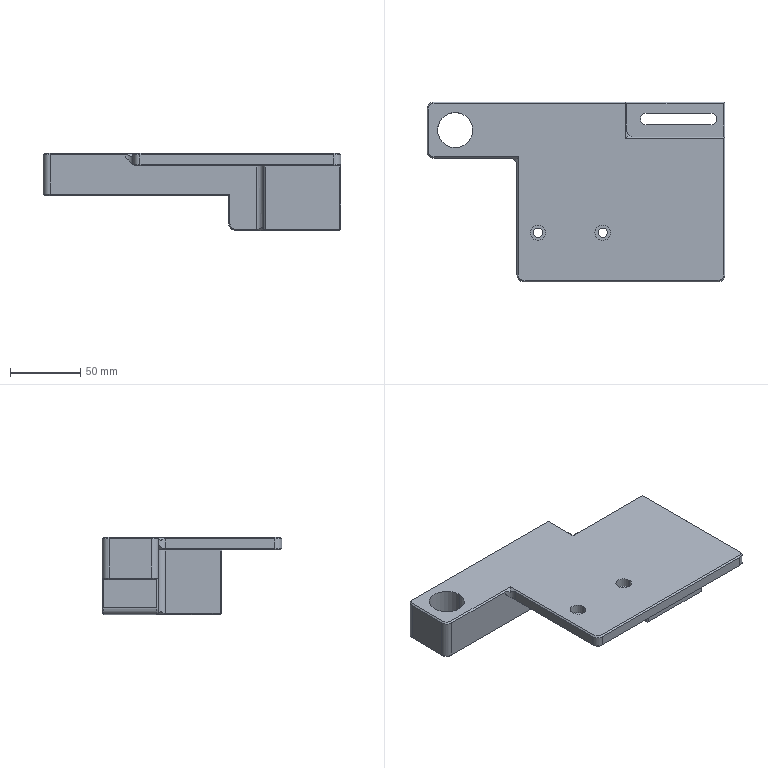NC program | NX | posted with a generic post | part box 212 x 128 x 55 mm
Lines 5359 to 7213 of 7327, first 1601 of 1847 lines:
(ZLEVEL_PROFILE_COPY_COPY_COPY , TOOL : D10)
N10674 T09 M6
N10676 G54
N10678 G17 G0 G90 X-48.2 Y14.719 S2000 M3
N10680 G43 Z30. H9
N10682 Z-0.2
N10684 G94 G1 X-46.7 Y15.585 F1000.
N10686 G3 X-46.2 Y16.451 R1.
N10688 G1 Y19.8 F2000.
N10690 X-49.549
N10692 G3 X-50.415 Y19.3 R1.
N10694 G1 X-51.281 Y17.8
N10696 G0 X-48.4 Y14.519 Z-0.4
N10698 G1 X-46.9 Y15.385 F1000.
N10700 G3 X-46.4 Y16.251 R1.
N10702 G1 Y19.6 F2000.
N10704 X-49.749
N10706 G3 X-50.615 Y19.1 R1.
N10708 G1 X-51.481 Y17.6
N10710 G0 X-48.6 Y14.319 Z-0.6
N10712 G1 X-47.1 Y15.185 F1000.
N10714 G3 X-46.6 Y16.051 R1.
N10716 G1 Y19.4 F2000.
N10718 X-49.949
N10720 G3 X-50.815 Y18.9 R1.
N10722 G1 X-51.681 Y17.4
N10724 G0 X-48.8 Y14.119 Z-0.8
N10726 G1 X-47.3 Y14.985 F1000.
N10728 G3 X-46.8 Y15.851 R1.
N10730 G1 Y19.2 F2000.
N10732 X-50.149
N10734 G3 X-51.015 Y18.7 R1.
N10736 G1 X-51.881 Y17.2
N10738 G0 X-49. Y13.919 Z-1.
N10740 G1 X-47.5 Y14.785 F1000.
N10742 G3 X-47. Y15.651 R1.
N10744 G1 Y19. F2000.
N10746 X-50.349
N10748 G3 X-51.215 Y18.5 R1.
N10750 G1 X-52.081 Y17.
N10752 G0 X-49. Y13.919 Z-1.2
N10754 G1 X-47.5 Y14.785 F1000.
N10756 G3 X-47. Y15.651 R1.
N10758 G1 Y18.956 F2000.
N10760 X-47.003 Y19.
N10762 X-50.349
N10764 G3 X-51.215 Y18.5 R1.
N10766 G1 X-52.081 Y17.
N10768 G0 X-49. Y13.919 Z-1.4
N10770 G1 X-47.5 Y14.785 F1000.
N10772 G3 X-47. Y15.651 R1.
N10774 G1 Y18.956 F2000.
N10776 X-47.003 Y19.
N10778 X-50.349
N10780 G3 X-51.215 Y18.5 R1.
N10782 G1 X-52.081 Y17.
N10784 G0 X-49. Y13.919 Z-1.6
N10786 G1 X-47.5 Y14.785 F1000.
N10788 G3 X-47. Y15.651 R1.
N10790 G1 Y18.956 F2000.
N10792 X-47.003 Y19.
N10794 X-50.349
N10796 G3 X-51.215 Y18.5 R1.
N10798 G1 X-52.081 Y17.
N10800 G0 X-49. Y13.919 Z-1.8
N10802 G1 X-47.5 Y14.785 F1000.
N10804 G3 X-47. Y15.651 R1.
N10806 G1 Y18.956 F2000.
N10808 X-47.003 Y19.
N10810 X-50.349
N10812 G3 X-51.215 Y18.5 R1.
N10814 G1 X-52.081 Y17.
N10816 G0 X-49. Y13.919 Z-2.
N10818 G1 X-47.5 Y14.785 F1000.
N10820 G3 X-47. Y15.651 R1.
N10822 G1 Y18.956 F2000.
N10824 X-47.003 Y19.
N10826 X-50.349
N10828 G3 X-51.215 Y18.5 R1.
N10830 G1 X-52.081 Y17.
N10832 G0 X-49. Y13.919 Z-2.2
N10834 G1 X-47.5 Y14.785 F1000.
N10836 G3 X-47. Y15.651 R1.
N10838 G1 Y18.956 F2000.
N10840 X-47.003 Y19.
N10842 X-50.349
N10844 G3 X-51.215 Y18.5 R1.
N10846 G1 X-52.081 Y17.
N10848 G0 X-49. Y13.919 Z-2.4
N10850 G1 X-47.5 Y14.785 F1000.
N10852 G3 X-47. Y15.651 R1.
N10854 G1 Y18.956 F2000.
N10856 X-47.003 Y19.
N10858 X-50.349
N10860 G3 X-51.215 Y18.5 R1.
N10862 G1 X-52.081 Y17.
N10864 G0 X-49. Y13.919 Z-2.6
N10866 G1 X-47.5 Y14.785 F1000.
N10868 G3 X-47. Y15.651 R1.
N10870 G1 Y18.956 F2000.
N10872 X-47.003 Y19.
N10874 X-50.349
N10876 G3 X-51.215 Y18.5 R1.
N10878 G1 X-52.081 Y17.
N10880 G0 X-49. Y13.919 Z-2.8
N10882 G1 X-47.5 Y14.785 F1000.
N10884 G3 X-47. Y15.651 R1.
N10886 G1 Y18.956 F2000.
N10888 X-47.003 Y19.
N10890 X-50.349
N10892 G3 X-51.215 Y18.5 R1.
N10894 G1 X-52.081 Y17.
N10896 G0 X-49. Y13.919 Z-3.
N10898 G1 X-47.5 Y14.785 F1000.
N10900 G3 X-47. Y15.651 R1.
N10902 G1 Y18.956 F2000.
N10904 X-47.003 Y19.
N10906 X-50.349
N10908 G3 X-51.215 Y18.5 R1.
N10910 G1 X-52.081 Y17.
N10912 G0 X-49. Y13.919 Z-3.2
N10914 G1 X-47.5 Y14.785 F1000.
N10916 G3 X-47. Y15.651 R1.
N10918 G1 Y19. F2000.
N10920 X-50.349
N10922 G3 X-51.215 Y18.5 R1.
N10924 G1 X-52.081 Y17.
N10926 G0 X-49. Y13.919 Z-3.4
N10928 G1 X-47.5 Y14.785 F1000.
N10930 G3 X-47. Y15.651 R1.
N10932 G1 Y19. F2000.
N10934 X-50.349
N10936 G3 X-51.215 Y18.5 R1.
N10938 G1 X-52.081 Y17.
N10940 G0 X-49. Y13.919 Z-3.6
N10942 G1 X-47.5 Y14.785 F1000.
N10944 G3 X-47. Y15.651 R1.
N10946 G1 Y19. F2000.
N10948 X-50.349
N10950 G3 X-51.215 Y18.5 R1.
N10952 G1 X-52.081 Y17.
N10954 G0 X-49. Y13.919 Z-3.8
N10956 G1 X-47.5 Y14.785 F1000.
N10958 G3 X-47. Y15.651 R1.
N10960 G1 Y19. F2000.
N10962 X-50.349
N10964 G3 X-51.215 Y18.5 R1.
N10966 G1 X-52.081 Y17.
N10968 G0 X-49. Y13.919 Z-4.
N10970 G1 X-47.5 Y14.785 F1000.
N10972 G3 X-47. Y15.651 R1.
N10974 G1 Y19. F2000.
N10976 X-50.349
N10978 G3 X-51.215 Y18.5 R1.
N10980 G1 X-52.081 Y17.
N10982 G0 X-49. Y13.919 Z-4.2
N10984 G1 X-47.5 Y14.785 F1000.
N10986 G3 X-47. Y15.651 R1.
N10988 G1 Y19. F2000.
N10990 X-50.349
N10992 G3 X-51.215 Y18.5 R1.
N10994 G1 X-52.081 Y17.
N10996 G0 X-49. Y13.919 Z-4.4
N10998 G1 X-47.5 Y14.785 F1000.
N11000 G3 X-47. Y15.651 R1.
N11002 G1 Y19. F2000.
N11004 X-50.349
N11006 G3 X-51.215 Y18.5 R1.
N11008 G1 X-52.081 Y17.
N11010 G0 X-49. Y13.919 Z-4.6
N11012 G1 X-47.5 Y14.785 F1000.
N11014 G3 X-47. Y15.651 R1.
N11016 G1 Y19. F2000.
N11018 X-50.349
N11020 G3 X-51.215 Y18.5 R1.
N11022 G1 X-52.081 Y17.
N11024 G0 X-49. Y13.919 Z-4.8
N11026 G1 X-47.5 Y14.785 F1000.
N11028 G3 X-47. Y15.651 R1.
N11030 G1 Y19. F2000.
N11032 X-50.349
N11034 G3 X-51.215 Y18.5 R1.
N11036 G1 X-52.081 Y17.
N11038 G0 X-49. Y13.919 Z-5.
N11040 G1 X-47.5 Y14.785 F1000.
N11042 G3 X-47. Y15.651 R1.
N11044 G1 Y19. F2000.
N11046 X-50.349
N11048 G3 X-51.215 Y18.5 R1.
N11050 G1 X-52.081 Y17.
N11052 G0 X-49. Y13.919 Z-5.2
N11054 G1 X-47.5 Y14.785 F1000.
N11056 G3 X-47. Y15.651 R1.
N11058 G1 Y19. F2000.
N11060 X-50.349
N11062 G3 X-51.215 Y18.5 R1.
N11064 G1 X-52.081 Y17.
N11066 G0 X-49. Y13.919 Z-5.4
N11068 G1 X-47.5 Y14.785 F1000.
N11070 G3 X-47. Y15.651 R1.
N11072 G1 Y19. F2000.
N11074 X-50.349
N11076 G3 X-51.215 Y18.5 R1.
N11078 G1 X-52.081 Y17.
N11080 G0 X-49. Y13.919 Z-5.6
N11082 G1 X-47.5 Y14.785 F1000.
N11084 G3 X-47. Y15.651 R1.
N11086 G1 Y19. F2000.
N11088 X-50.349
N11090 G3 X-51.215 Y18.5 R1.
N11092 G1 X-52.081 Y17.
N11094 G0 X-49. Y13.919 Z-5.8
N11096 G1 X-47.5 Y14.785 F1000.
N11098 G3 X-47. Y15.651 R1.
N11100 G1 Y19. F2000.
N11102 X-50.349
N11104 G3 X-51.215 Y18.5 R1.
N11106 G1 X-52.081 Y17.
N11108 G0 X-49. Y13.919 Z-6.
N11110 G1 X-47.5 Y14.785 F1000.
N11112 G3 X-47. Y15.651 R1.
N11114 G1 Y19. F2000.
N11116 X-50.349
N11118 G3 X-51.215 Y18.5 R1.
N11120 G1 X-52.081 Y17.
N11122 G0 X-49. Y13.919 Z-6.2
N11124 G1 X-47.5 Y14.785 F1000.
N11126 G3 X-47. Y15.651 R1.
N11128 G1 Y19. F2000.
N11130 X-50.349
N11132 G3 X-51.215 Y18.5 R1.
N11134 G1 X-52.081 Y17.
N11136 G0 X-49. Y13.919 Z-6.4
N11138 G1 X-47.5 Y14.785 F1000.
N11140 G3 X-47. Y15.651 R1.
N11142 G1 Y19. F2000.
N11144 X-50.349
N11146 G3 X-51.215 Y18.5 R1.
N11148 G1 X-52.081 Y17.
N11150 G0 X-49. Y13.919 Z-6.6
N11152 G1 X-47.5 Y14.785 F1000.
N11154 G3 X-47. Y15.651 R1.
N11156 G1 Y19. F2000.
N11158 X-50.349
N11160 G3 X-51.215 Y18.5 R1.
N11162 G1 X-52.081 Y17.
N11164 G0 X-49. Y13.919 Z-6.8
N11166 G1 X-47.5 Y14.785 F1000.
N11168 G3 X-47. Y15.651 R1.
N11170 G1 Y19. F2000.
N11172 X-50.349
N11174 G3 X-51.215 Y18.5 R1.
N11176 G1 X-52.081 Y17.
N11178 G0 X-49. Y13.919 Z-7.
N11180 G1 X-47.5 Y14.785 F1000.
N11182 G3 X-47. Y15.651 R1.
N11184 G1 Y19. F2000.
N11186 X-50.349
N11188 G3 X-51.215 Y18.5 R1.
N11190 G1 X-52.081 Y17.
N11192 G0 X-49. Y13.919 Z-7.2
N11194 G1 X-47.5 Y14.785 F1000.
N11196 G3 X-47. Y15.651 R1.
N11198 G1 Y19. F2000.
N11200 X-50.349
N11202 G3 X-51.215 Y18.5 R1.
N11204 G1 X-52.081 Y17.
N11206 G0 X-49. Y13.919 Z-7.4
N11208 G1 X-47.5 Y14.785 F1000.
N11210 G3 X-47. Y15.651 R1.
N11212 G1 Y19. F2000.
N11214 X-50.349
N11216 G3 X-51.215 Y18.5 R1.
N11218 G1 X-52.081 Y17.
N11220 G0 X-49. Y13.919 Z-7.6
N11222 G1 X-47.5 Y14.785 F1000.
N11224 G3 X-47. Y15.651 R1.
N11226 G1 Y19. F2000.
N11228 X-50.349
N11230 G3 X-51.215 Y18.5 R1.
N11232 G1 X-52.081 Y17.
N11234 G0 X-49. Y13.919 Z-7.8
N11236 G1 X-47.5 Y14.785 F1000.
N11238 G3 X-47. Y15.651 R1.
N11240 G1 Y19. F2000.
N11242 X-50.349
N11244 G3 X-51.215 Y18.5 R1.
N11246 G1 X-52.081 Y17.
N11248 G0 X-49. Y13.919 Z-8.
N11250 G1 X-47.5 Y14.785 F1000.
N11252 G3 X-47. Y15.651 R1.
N11254 G1 Y19. F2000.
N11256 X-50.349
N11258 G3 X-51.215 Y18.5 R1.
N11260 G1 X-52.081 Y17.
N11262 G0 X-49. Y13.919 Z-8.2
N11264 G1 X-47.5 Y14.785 F1000.
N11266 G3 X-47. Y15.651 R1.
N11268 G1 Y19. F2000.
N11270 X-50.349
N11272 G3 X-51.215 Y18.5 R1.
N11274 G1 X-52.081 Y17.
N11276 G0 X-49. Y13.919 Z-8.4
N11278 G1 X-47.5 Y14.785 F1000.
N11280 G3 X-47. Y15.651 R1.
N11282 G1 Y19. F2000.
N11284 X-50.349
N11286 G3 X-51.215 Y18.5 R1.
N11288 G1 X-52.081 Y17.
N11290 G0 X-49. Y13.919 Z-8.6
N11292 G1 X-47.5 Y14.785 F1000.
N11294 G3 X-47. Y15.651 R1.
N11296 G1 Y19. F2000.
N11298 X-50.349
N11300 G3 X-51.215 Y18.5 R1.
N11302 G1 X-52.081 Y17.
N11304 G0 X-49. Y13.919 Z-8.8
N11306 G1 X-47.5 Y14.785 F1000.
N11308 G3 X-47. Y15.651 R1.
N11310 G1 Y19. F2000.
N11312 X-50.349
N11314 G3 X-51.215 Y18.5 R1.
N11316 G1 X-52.081 Y17.
N11318 G0 X-49. Y13.919 Z-9.
N11320 G1 X-47.5 Y14.785 F1000.
N11322 G3 X-47. Y15.651 R1.
N11324 G1 Y19. F2000.
N11326 X-50.349
N11328 G3 X-51.215 Y18.5 R1.
N11330 G1 X-52.081 Y17.
N11332 G0 Z30.
N11334 X42.2 Y48.281
N11336 Z-0.2
N11338 G1 X40.7 Y47.415 F1000.
N11340 G3 X40.2 Y46.549 R1.
N11342 G1 Y43.2 F2000.
N11344 X43.549
N11346 G3 X44.415 Y43.7 R1.
N11348 G1 X45.281 Y45.2
N11350 G0 X42.4 Y48.481 Z-0.4
N11352 G1 X40.9 Y47.615 F1000.
N11354 G3 X40.4 Y46.749 R1.
N11356 G1 Y43.4 F2000.
N11358 X43.749
N11360 G3 X44.615 Y43.9 R1.
N11362 G1 X45.481 Y45.4
N11364 G0 X42.6 Y48.681 Z-0.6
N11366 G1 X41.1 Y47.815 F1000.
N11368 G3 X40.6 Y46.949 R1.
N11370 G1 Y43.6 F2000.
N11372 X43.949
N11374 G3 X44.815 Y44.1 R1.
N11376 G1 X45.681 Y45.6
N11378 G0 X42.8 Y48.881 Z-0.8
N11380 G1 X41.3 Y48.015 F1000.
N11382 G3 X40.8 Y47.149 R1.
N11384 G1 Y43.8 F2000.
N11386 X44.149
N11388 G3 X45.015 Y44.3 R1.
N11390 G1 X45.881 Y45.8
N11392 G0 X43. Y49.081 Z-1.
N11394 G1 X41.5 Y48.215 F1000.
N11396 G3 X41. Y47.349 R1.
N11398 G1 Y44. F2000.
N11400 X44.349
N11402 G3 X45.215 Y44.5 R1.
N11404 G1 X46.081 Y46.
N11406 G0 X43. Y49.081 Z-1.2
N11408 G1 X41.5 Y48.215 F1000.
N11410 G3 X41. Y47.349 R1.
N11412 G1 Y44. F2000.
N11414 X44.349
N11416 G3 X45.215 Y44.5 R1.
N11418 G1 X46.081 Y46.
N11420 G0 X43. Y49.081 Z-1.4
N11422 G1 X41.5 Y48.215 F1000.
N11424 G3 X41. Y47.349 R1.
N11426 G1 Y44. F2000.
N11428 X44.349
N11430 G3 X45.215 Y44.5 R1.
N11432 G1 X46.081 Y46.
N11434 G0 X43. Y49.081 Z-1.6
N11436 G1 X41.5 Y48.215 F1000.
N11438 G3 X41. Y47.349 R1.
N11440 G1 Y44. F2000.
N11442 X44.349
N11444 G3 X45.215 Y44.5 R1.
N11446 G1 X46.081 Y46.
N11448 G0 X43. Y49.081 Z-1.8
N11450 G1 X41.5 Y48.215 F1000.
N11452 G3 X41. Y47.349 R1.
N11454 G1 Y44. F2000.
N11456 X44.349
N11458 G3 X45.215 Y44.5 R1.
N11460 G1 X46.081 Y46.
N11462 G0 X43. Y49.081 Z-2.
N11464 G1 X41.5 Y48.215 F1000.
N11466 G3 X41. Y47.349 R1.
N11468 G1 Y44. F2000.
N11470 X44.349
N11472 G3 X45.215 Y44.5 R1.
N11474 G1 X46.081 Y46.
N11476 G0 X43. Y49.081 Z-2.2
N11478 G1 X41.5 Y48.215 F1000.
N11480 G3 X41. Y47.349 R1.
N11482 G1 Y44. F2000.
N11484 X44.349
N11486 G3 X45.215 Y44.5 R1.
N11488 G1 X46.081 Y46.
N11490 G0 X43. Y49.081 Z-2.4
N11492 G1 X41.5 Y48.215 F1000.
N11494 G3 X41. Y47.349 R1.
N11496 G1 Y44. F2000.
N11498 X44.349
N11500 G3 X45.215 Y44.5 R1.
N11502 G1 X46.081 Y46.
N11504 G0 X43. Y49.081 Z-2.6
N11506 G1 X41.5 Y48.215 F1000.
N11508 G3 X41. Y47.349 R1.
N11510 G1 Y44. F2000.
N11512 X44.349
N11514 G3 X45.215 Y44.5 R1.
N11516 G1 X46.081 Y46.
N11518 G0 X43. Y49.081 Z-2.8
N11520 G1 X41.5 Y48.215 F1000.
N11522 G3 X41. Y47.349 R1.
N11524 G1 Y44. F2000.
N11526 X44.349
N11528 G3 X45.215 Y44.5 R1.
N11530 G1 X46.081 Y46.
N11532 G0 X43. Y49.081 Z-3.
N11534 G1 X41.5 Y48.215 F1000.
N11536 G3 X41. Y47.349 R1.
N11538 G1 Y44. F2000.
N11540 X44.349
N11542 G3 X45.215 Y44.5 R1.
N11544 G1 X46.081 Y46.
N11546 G0 X43. Y49.081 Z-3.2
N11548 G1 X41.5 Y48.215 F1000.
N11550 G3 X41. Y47.349 R1.
N11552 G1 Y44. F2000.
N11554 X44.349
N11556 G3 X45.215 Y44.5 R1.
N11558 G1 X46.081 Y46.
N11560 G0 X43. Y49.081 Z-3.4
N11562 G1 X41.5 Y48.215 F1000.
N11564 G3 X41. Y47.349 R1.
N11566 G1 Y44. F2000.
N11568 X44.349
N11570 G3 X45.215 Y44.5 R1.
N11572 G1 X46.081 Y46.
N11574 G0 X43. Y49.081 Z-3.6
N11576 G1 X41.5 Y48.215 F1000.
N11578 G3 X41. Y47.349 R1.
N11580 G1 Y44. F2000.
N11582 X44.349
N11584 G3 X45.215 Y44.5 R1.
N11586 G1 X46.081 Y46.
N11588 G0 X43. Y49.081 Z-3.8
N11590 G1 X41.5 Y48.215 F1000.
N11592 G3 X41. Y47.349 R1.
N11594 G1 Y44. F2000.
N11596 X44.349
N11598 G3 X45.215 Y44.5 R1.
N11600 G1 X46.081 Y46.
N11602 G0 X43. Y49.081 Z-4.
N11604 G1 X41.5 Y48.215 F1000.
N11606 G3 X41. Y47.349 R1.
N11608 G1 Y44. F2000.
N11610 X44.349
N11612 G3 X45.215 Y44.5 R1.
N11614 G1 X46.081 Y46.
N11616 G0 X43. Y49.081 Z-4.2
N11618 G1 X41.5 Y48.215 F1000.
N11620 G3 X41. Y47.349 R1.
N11622 G1 Y44. F2000.
N11624 X44.349
N11626 G3 X45.215 Y44.5 R1.
N11628 G1 X46.081 Y46.
N11630 G0 X43. Y49.081 Z-4.4
N11632 G1 X41.5 Y48.215 F1000.
N11634 G3 X41. Y47.349 R1.
N11636 G1 Y44. F2000.
N11638 X44.349
N11640 G3 X45.215 Y44.5 R1.
N11642 G1 X46.081 Y46.
N11644 G0 X43. Y49.081 Z-4.6
N11646 G1 X41.5 Y48.215 F1000.
N11648 G3 X41. Y47.349 R1.
N11650 G1 Y44. F2000.
N11652 X44.349
N11654 G3 X45.215 Y44.5 R1.
N11656 G1 X46.081 Y46.
N11658 G0 X43. Y49.081 Z-4.8
N11660 G1 X41.5 Y48.215 F1000.
N11662 G3 X41. Y47.349 R1.
N11664 G1 Y44. F2000.
N11666 X44.349
N11668 G3 X45.215 Y44.5 R1.
N11670 G1 X46.081 Y46.
N11672 G0 X43. Y49.081 Z-5.
N11674 G1 X41.5 Y48.215 F1000.
N11676 G3 X41. Y47.349 R1.
N11678 G1 Y44. F2000.
N11680 X44.349
N11682 G3 X45.215 Y44.5 R1.
N11684 G1 X46.081 Y46.
N11686 G0 X43. Y49.081 Z-5.2
N11688 G1 X41.5 Y48.215 F1000.
N11690 G3 X41. Y47.349 R1.
N11692 G1 Y44. F2000.
N11694 X44.349
N11696 G3 X45.215 Y44.5 R1.
N11698 G1 X46.081 Y46.
N11700 G0 X43. Y49.081 Z-5.4
N11702 G1 X41.5 Y48.215 F1000.
N11704 G3 X41. Y47.349 R1.
N11706 G1 Y44. F2000.
N11708 X44.349
N11710 G3 X45.215 Y44.5 R1.
N11712 G1 X46.081 Y46.
N11714 G0 X43. Y49.081 Z-5.6
N11716 G1 X41.5 Y48.215 F1000.
N11718 G3 X41. Y47.349 R1.
N11720 G1 Y44. F2000.
N11722 X44.349
N11724 G3 X45.215 Y44.5 R1.
N11726 G1 X46.081 Y46.
N11728 G0 X43. Y49.081 Z-5.8
N11730 G1 X41.5 Y48.215 F1000.
N11732 G3 X41. Y47.349 R1.
N11734 G1 Y44. F2000.
N11736 X44.349
N11738 G3 X45.215 Y44.5 R1.
N11740 G1 X46.081 Y46.
N11742 G0 X43. Y49.081 Z-6.
N11744 G1 X41.5 Y48.215 F1000.
N11746 G3 X41. Y47.349 R1.
N11748 G1 Y44. F2000.
N11750 X44.349
N11752 G3 X45.215 Y44.5 R1.
N11754 G1 X46.081 Y46.
N11756 G0 X43. Y49.081 Z-6.2
N11758 G1 X41.5 Y48.215 F1000.
N11760 G3 X41. Y47.349 R1.
N11762 G1 Y44. F2000.
N11764 X44.349
N11766 G3 X45.215 Y44.5 R1.
N11768 G1 X46.081 Y46.
N11770 G0 X43. Y49.081 Z-6.4
N11772 G1 X41.5 Y48.215 F1000.
N11774 G3 X41. Y47.349 R1.
N11776 G1 Y44. F2000.
N11778 X44.349
N11780 G3 X45.215 Y44.5 R1.
N11782 G1 X46.081 Y46.
N11784 G0 X43. Y49.081 Z-6.6
N11786 G1 X41.5 Y48.215 F1000.
N11788 G3 X41. Y47.349 R1.
N11790 G1 Y44. F2000.
N11792 X44.349
N11794 G3 X45.215 Y44.5 R1.
N11796 G1 X46.081 Y46.
N11798 G0 X43. Y49.081 Z-6.8
N11800 G1 X41.5 Y48.215 F1000.
N11802 G3 X41. Y47.349 R1.
N11804 G1 Y44. F2000.
N11806 X44.349
N11808 G3 X45.215 Y44.5 R1.
N11810 G1 X46.081 Y46.
N11812 G0 X43. Y49.081 Z-7.
N11814 G1 X41.5 Y48.215 F1000.
N11816 G3 X41. Y47.349 R1.
N11818 G1 Y44. F2000.
N11820 X44.349
N11822 G3 X45.215 Y44.5 R1.
N11824 G1 X46.081 Y46.
N11826 G0 X43. Y49.081 Z-7.2
N11828 G1 X41.5 Y48.215 F1000.
N11830 G3 X41. Y47.349 R1.
N11832 G1 Y44. F2000.
N11834 X44.349
N11836 G3 X45.215 Y44.5 R1.
N11838 G1 X46.081 Y46.
N11840 G0 X43. Y49.081 Z-7.4
N11842 G1 X41.5 Y48.215 F1000.
N11844 G3 X41. Y47.349 R1.
N11846 G1 Y44. F2000.
N11848 X44.349
N11850 G3 X45.215 Y44.5 R1.
N11852 G1 X46.081 Y46.
N11854 G0 X43. Y49.081 Z-7.6
N11856 G1 X41.5 Y48.215 F1000.
N11858 G3 X41. Y47.349 R1.
N11860 G1 Y44. F2000.
N11862 X44.349
N11864 G3 X45.215 Y44.5 R1.
N11866 G1 X46.081 Y46.
N11868 G0 X43. Y49.081 Z-7.8
N11870 G1 X41.5 Y48.215 F1000.
N11872 G3 X41. Y47.349 R1.
N11874 G1 Y44. F2000.
N11876 X44.349
N11878 G3 X45.215 Y44.5 R1.
N11880 G1 X46.081 Y46.
N11882 G0 X43. Y49.081 Z-8.
N11884 G1 X41.5 Y48.215 F1000.
N11886 G3 X41. Y47.349 R1.
N11888 G1 Y44. F2000.
N11890 X44.349
N11892 G3 X45.215 Y44.5 R1.
N11894 G1 X46.081 Y46.
N11896 G0 X43. Y49.081 Z-8.2
N11898 G1 X41.5 Y48.215 F1000.
N11900 G3 X41. Y47.349 R1.
N11902 G1 Y44. F2000.
N11904 X44.349
N11906 G3 X45.215 Y44.5 R1.
N11908 G1 X46.081 Y46.
N11910 G0 X43. Y49.081 Z-8.4
N11912 G1 X41.5 Y48.215 F1000.
N11914 G3 X41. Y47.349 R1.
N11916 G1 Y44. F2000.
N11918 X44.349
N11920 G3 X45.215 Y44.5 R1.
N11922 G1 X46.081 Y46.
N11924 G0 X43. Y49.081 Z-8.6
N11926 G1 X41.5 Y48.215 F1000.
N11928 G3 X41. Y47.349 R1.
N11930 G1 Y44. F2000.
N11932 X44.349
N11934 G3 X45.215 Y44.5 R1.
N11936 G1 X46.081 Y46.
N11938 G0 X43. Y49.081 Z-8.8
N11940 G1 X41.5 Y48.215 F1000.
N11942 G3 X41. Y47.349 R1.
N11944 G1 Y44. F2000.
N11946 X44.349
N11948 G3 X45.215 Y44.5 R1.
N11950 G1 X46.081 Y46.
N11952 G0 X43. Y49.081 Z-9.
N11954 G1 X41.5 Y48.215 F1000.
N11956 G3 X41. Y47.349 R1.
N11958 G1 Y44. F2000.
N11960 X44.349
N11962 G3 X45.215 Y44.5 R1.
N11964 G1 X46.081 Y46.
N11966 G0 X43. Y49.081 Z-9.2
N11968 G1 X41.5 Y48.215 F1000.
N11970 G3 X41. Y47.349 R1.
N11972 G1 Y44. F2000.
N11974 X44.349
N11976 G3 X45.215 Y44.5 R1.
N11978 G1 X46.081 Y46.
N11980 G0 X43. Y49.081 Z-9.4
N11982 G1 X41.5 Y48.215 F1000.
N11984 G3 X41. Y47.349 R1.
N11986 G1 Y44. F2000.
N11988 X44.349
N11990 G3 X45.215 Y44.5 R1.
N11992 G1 X46.081 Y46.
N11994 G0 X43. Y49.081 Z-9.6
N11996 G1 X41.5 Y48.215 F1000.
N11998 G3 X41. Y47.349 R1.
N12000 G1 Y44. F2000.
N12002 X44.349
N12004 G3 X45.215 Y44.5 R1.
N12006 G1 X46.081 Y46.
N12008 G0 X43. Y49.081 Z-9.8
N12010 G1 X41.5 Y48.215 F1000.
N12012 G3 X41. Y47.349 R1.
N12014 G1 Y44. F2000.
N12016 X44.349
N12018 G3 X45.215 Y44.5 R1.
N12020 G1 X46.081 Y46.
N12022 G0 X43. Y49.081 Z-10.
N12024 G1 X41.5 Y48.215 F1000.
N12026 G3 X41. Y47.349 R1.
N12028 G1 Y44. F2000.
N12030 X44.349
N12032 G3 X45.215 Y44.5 R1.
N12034 G1 X46.081 Y46.
N12036 G0 X43. Y49.081 Z-10.2
N12038 G1 X41.5 Y48.215 F1000.
N12040 G3 X41. Y47.349 R1.
N12042 G1 Y44. F2000.
N12044 X44.349
N12046 G3 X45.215 Y44.5 R1.
N12048 G1 X46.081 Y46.
N12050 G0 X43. Y49.081 Z-10.4
N12052 G1 X41.5 Y48.215 F1000.
N12054 G3 X41. Y47.349 R1.
N12056 G1 Y44. F2000.
N12058 X44.349
N12060 G3 X45.215 Y44.5 R1.
N12062 G1 X46.081 Y46.
N12064 G0 X43. Y49.081 Z-10.6
N12066 G1 X41.5 Y48.215 F1000.
N12068 G3 X41. Y47.349 R1.
N12070 G1 Y44. F2000.
N12072 X44.349
N12074 G3 X45.215 Y44.5 R1.
N12076 G1 X46.081 Y46.
N12078 G0 X43. Y49.081 Z-10.8
N12080 G1 X41.5 Y48.215 F1000.
N12082 G3 X41. Y47.349 R1.
N12084 G1 Y44. F2000.
N12086 X44.349
N12088 G3 X45.215 Y44.5 R1.
N12090 G1 X46.081 Y46.
N12092 G0 X43. Y49.081 Z-11.
N12094 G1 X41.5 Y48.215 F1000.
N12096 G3 X41. Y47.349 R1.
N12098 G1 Y44. F2000.
N12100 X44.349
N12102 G3 X45.215 Y44.5 R1.
N12104 G1 X46.081 Y46.
N12106 G0 X43. Y49.081 Z-11.2
N12108 G1 X41.5 Y48.215 F1000.
N12110 G3 X41. Y47.349 R1.
N12112 G1 Y44. F2000.
N12114 X44.349
N12116 G3 X45.215 Y44.5 R1.
N12118 G1 X46.081 Y46.
N12120 G0 X43. Y49.081 Z-11.4
N12122 G1 X41.5 Y48.215 F1000.
N12124 G3 X41. Y47.349 R1.
N12126 G1 Y44. F2000.
N12128 X44.349
N12130 G3 X45.215 Y44.5 R1.
N12132 G1 X46.081 Y46.
N12134 G0 X43. Y49.081 Z-11.6
N12136 G1 X41.5 Y48.215 F1000.
N12138 G3 X41. Y47.349 R1.
N12140 G1 Y44. F2000.
N12142 X44.349
N12144 G3 X45.215 Y44.5 R1.
N12146 G1 X46.081 Y46.
N12148 G0 X43. Y49.081 Z-11.8
N12150 G1 X41.5 Y48.215 F1000.
N12152 G3 X41. Y47.349 R1.
N12154 G1 Y44. F2000.
N12156 X44.349
N12158 G3 X45.215 Y44.5 R1.
N12160 G1 X46.081 Y46.
N12162 G0 X43. Y49.081 Z-12.
N12164 G1 X41.5 Y48.215 F1000.
N12166 G3 X41. Y47.349 R1.
N12168 G1 Y44. F2000.
N12170 X44.349
N12172 G3 X45.215 Y44.5 R1.
N12174 G1 X46.081 Y46.
N12176 G0 X43. Y49.081 Z-12.2
N12178 G1 X41.5 Y48.215 F1000.
N12180 G3 X41. Y47.349 R1.
N12182 G1 Y44. F2000.
N12184 X44.349
N12186 G3 X45.215 Y44.5 R1.
N12188 G1 X46.081 Y46.
N12190 G0 X43. Y49.081 Z-12.4
N12192 G1 X41.5 Y48.215 F1000.
N12194 G3 X41. Y47.349 R1.
N12196 G1 Y44. F2000.
N12198 X44.349
N12200 G3 X45.215 Y44.5 R1.
N12202 G1 X46.081 Y46.
N12204 G0 X43. Y49.081 Z-12.6
N12206 G1 X41.5 Y48.215 F1000.
N12208 G3 X41. Y47.349 R1.
N12210 G1 Y44. F2000.
N12212 X44.349
N12214 G3 X45.215 Y44.5 R1.
N12216 G1 X46.081 Y46.
N12218 G0 X43. Y49.081 Z-12.8
N12220 G1 X41.5 Y48.215 F1000.
N12222 G3 X41. Y47.349 R1.
N12224 G1 Y44. F2000.
N12226 X44.349
N12228 G3 X45.215 Y44.5 R1.
N12230 G1 X46.081 Y46.
N12232 G0 X43. Y49.081 Z-13.
N12234 G1 X41.5 Y48.215 F1000.
N12236 G3 X41. Y47.349 R1.
N12238 G1 Y44. F2000.
N12240 X44.349
N12242 G3 X45.215 Y44.5 R1.
N12244 G1 X46.081 Y46.
N12246 G0 X43. Y49.081 Z-13.2
N12248 G1 X41.5 Y48.215 F1000.
N12250 G3 X41. Y47.349 R1.
N12252 G1 Y44. F2000.
N12254 X44.349
N12256 G3 X45.215 Y44.5 R1.
N12258 G1 X46.081 Y46.
N12260 G0 X43. Y49.081 Z-13.4
N12262 G1 X41.5 Y48.215 F1000.
N12264 G3 X41. Y47.349 R1.
N12266 G1 Y44. F2000.
N12268 X44.349
N12270 G3 X45.215 Y44.5 R1.
N12272 G1 X46.081 Y46.
N12274 G0 X43. Y49.081 Z-13.6
N12276 G1 X41.5 Y48.215 F1000.
N12278 G3 X41. Y47.349 R1.
N12280 G1 Y44. F2000.
N12282 X44.349
N12284 G3 X45.215 Y44.5 R1.
N12286 G1 X46.081 Y46.
N12288 G0 X43. Y49.081 Z-13.8
N12290 G1 X41.5 Y48.215 F1000.
N12292 G3 X41. Y47.349 R1.
N12294 G1 Y44. F2000.
N12296 X44.349
N12298 G3 X45.215 Y44.5 R1.
N12300 G1 X46.081 Y46.
N12302 G0 X43. Y49.081 Z-14.
N12304 G1 X41.5 Y48.215 F1000.
N12306 G3 X41. Y47.349 R1.
N12308 G1 Y44. F2000.
N12310 X44.349
N12312 G3 X45.215 Y44.5 R1.
N12314 G1 X46.081 Y46.
N12316 G0 X43. Y49.081 Z-14.2
N12318 G1 X41.5 Y48.215 F1000.
N12320 G3 X41. Y47.349 R1.
N12322 G1 Y44. F2000.
N12324 X44.349
N12326 G3 X45.215 Y44.5 R1.
N12328 G1 X46.081 Y46.
N12330 G0 X43. Y49.081 Z-14.4
N12332 G1 X41.5 Y48.215 F1000.
N12334 G3 X41. Y47.349 R1.
N12336 G1 Y44. F2000.
N12338 X44.349
N12340 G3 X45.215 Y44.5 R1.
N12342 G1 X46.081 Y46.
N12344 G0 X43. Y49.081 Z-14.6
N12346 G1 X41.5 Y48.215 F1000.
N12348 G3 X41. Y47.349 R1.
N12350 G1 Y44. F2000.
N12352 X44.349
N12354 G3 X45.215 Y44.5 R1.
N12356 G1 X46.081 Y46.
N12358 G0 X43. Y49.081 Z-14.8
N12360 G1 X41.5 Y48.215 F1000.
N12362 G3 X41. Y47.349 R1.
N12364 G1 Y44. F2000.
N12366 X44.349
N12368 G3 X45.215 Y44.5 R1.
N12370 G1 X46.081 Y46.
N12372 G0 X43. Y49.081 Z-15.
N12374 G1 X41.5 Y48.215 F1000.
N12376 G3 X41. Y47.349 R1.
N12378 G1 Y44. F2000.
N12380 X44.349
N12382 G3 X45.215 Y44.5 R1.
N12384 G1 X46.081 Y46.
N12386 G0 X43. Y49.081 Z-15.2
N12388 G1 X41.5 Y48.215 F1000.
N12390 G3 X41. Y47.349 R1.
N12392 G1 Y44. F2000.
N12394 X44.349
N12396 G3 X45.215 Y44.5 R1.
N12398 G1 X46.081 Y46.
N12400 G0 X43. Y49.081 Z-15.4
N12402 G1 X41.5 Y48.215 F1000.
N12404 G3 X41. Y47.349 R1.
N12406 G1 Y44. F2000.
N12408 X44.349
N12410 G3 X45.215 Y44.5 R1.
N12412 G1 X46.081 Y46.
N12414 G0 X43. Y49.081 Z-15.6
N12416 G1 X41.5 Y48.215 F1000.
N12418 G3 X41. Y47.349 R1.
N12420 G1 Y44. F2000.
N12422 X44.349
N12424 G3 X45.215 Y44.5 R1.
N12426 G1 X46.081 Y46.
N12428 G0 X43. Y49.081 Z-15.8
N12430 G1 X41.5 Y48.215 F1000.
N12432 G3 X41. Y47.349 R1.
N12434 G1 Y44. F2000.
N12436 X44.349
N12438 G3 X45.215 Y44.5 R1.
N12440 G1 X46.081 Y46.
N12442 G0 X43. Y49.081 Z-16.
N12444 G1 X41.5 Y48.215 F1000.
N12446 G3 X41. Y47.349 R1.
N12448 G1 Y44. F2000.
N12450 X44.349
N12452 G3 X45.215 Y44.5 R1.
N12454 G1 X46.081 Y46.
N12456 G0 X43. Y49.081 Z-16.2
N12458 G1 X41.5 Y48.215 F1000.
N12460 G3 X41. Y47.349 R1.
N12462 G1 Y44. F2000.
N12464 X44.349
N12466 G3 X45.215 Y44.5 R1.
N12468 G1 X46.081 Y46.
N12470 G0 X43. Y49.081 Z-16.4
N12472 G1 X41.5 Y48.215 F1000.
N12474 G3 X41. Y47.349 R1.
N12476 G1 Y44. F2000.
N12478 X44.349
N12480 G3 X45.215 Y44.5 R1.
N12482 G1 X46.081 Y46.
N12484 G0 X43. Y49.081 Z-16.6
N12486 G1 X41.5 Y48.215 F1000.
N12488 G3 X41. Y47.349 R1.
N12490 G1 Y44. F2000.
N12492 X44.349
N12494 G3 X45.215 Y44.5 R1.
N12496 G1 X46.081 Y46.
N12498 G0 X43. Y49.081 Z-16.8
N12500 G1 X41.5 Y48.215 F1000.
N12502 G3 X41. Y47.349 R1.
N12504 G1 Y44. F2000.
N12506 X44.349
N12508 G3 X45.215 Y44.5 R1.
N12510 G1 X46.081 Y46.
N12512 G0 X43. Y49.081 Z-17.
N12514 G1 X41.5 Y48.215 F1000.
N12516 G3 X41. Y47.349 R1.
N12518 G1 Y44. F2000.
N12520 X44.349
N12522 G3 X45.215 Y44.5 R1.
N12524 G1 X46.081 Y46.
N12526 G0 X43. Y49.081 Z-17.2
N12528 G1 X41.5 Y48.215 F1000.
N12530 G3 X41. Y47.349 R1.
N12532 G1 Y44. F2000.
N12534 X44.349
N12536 G3 X45.215 Y44.5 R1.
N12538 G1 X46.081 Y46.
N12540 G0 X43. Y49.081 Z-17.4
N12542 G1 X41.5 Y48.215 F1000.
N12544 G3 X41. Y47.349 R1.
N12546 G1 Y44. F2000.
N12548 X44.349
N12550 G3 X45.215 Y44.5 R1.
N12552 G1 X46.081 Y46.
N12554 G0 X43. Y49.081 Z-17.6
N12556 G1 X41.5 Y48.215 F1000.
N12558 G3 X41. Y47.349 R1.
N12560 G1 Y44. F2000.
N12562 X44.349
N12564 G3 X45.215 Y44.5 R1.
N12566 G1 X46.081 Y46.
N12568 G0 X43. Y49.081 Z-17.8
N12570 G1 X41.5 Y48.215 F1000.
N12572 G3 X41. Y47.349 R1.
N12574 G1 Y44. F2000.
N12576 X44.349
N12578 G3 X45.215 Y44.5 R1.
N12580 G1 X46.081 Y46.
N12582 G0 X43. Y49.081 Z-18.
N12584 G1 X41.5 Y48.215 F1000.
N12586 G3 X41. Y47.349 R1.
N12588 G1 Y44. F2000.
N12590 X44.349
N12592 G3 X45.215 Y44.5 R1.
N12594 G1 X46.081 Y46.
N12596 G0 X43. Y49.081 Z-18.2
N12598 G1 X41.5 Y48.215 F1000.
N12600 G3 X41. Y47.349 R1.
N12602 G1 Y44. F2000.
N12604 X44.349
N12606 G3 X45.215 Y44.5 R1.
N12608 G1 X46.081 Y46.
N12610 G0 X43. Y49.081 Z-18.4
N12612 G1 X41.5 Y48.215 F1000.
N12614 G3 X41. Y47.349 R1.
N12616 G1 Y44. F2000.
N12618 X44.349
N12620 G3 X45.215 Y44.5 R1.
N12622 G1 X46.081 Y46.
N12624 G0 X43. Y49.081 Z-18.6
N12626 G1 X41.5 Y48.215 F1000.
N12628 G3 X41. Y47.349 R1.
N12630 G1 Y44. F2000.
N12632 X44.349
N12634 G3 X45.215 Y44.5 R1.
N12636 G1 X46.081 Y46.
N12638 G0 X43. Y49.081 Z-18.8
N12640 G1 X41.5 Y48.215 F1000.
N12642 G3 X41. Y47.349 R1.
N12644 G1 Y44. F2000.
N12646 X44.349
N12648 G3 X45.215 Y44.5 R1.
N12650 G1 X46.081 Y46.
N12652 G0 X43. Y49.081 Z-19.
N12654 G1 X41.5 Y48.215 F1000.
N12656 G3 X41. Y47.349 R1.
N12658 G1 Y44. F2000.
N12660 X44.349
N12662 G3 X45.215 Y44.5 R1.
N12664 G1 X46.081 Y46.
N12666 G0 X43. Y49.081 Z-19.2
N12668 G1 X41.5 Y48.215 F1000.
N12670 G3 X41. Y47.349 R1.
N12672 G1 Y44. F2000.
N12674 X44.349
N12676 G3 X45.215 Y44.5 R1.
N12678 G1 X46.081 Y46.
N12680 G0 X43. Y49.081 Z-19.4
N12682 G1 X41.5 Y48.215 F1000.
N12684 G3 X41. Y47.349 R1.
N12686 G1 Y44. F2000.
N12688 X44.349
N12690 G3 X45.215 Y44.5 R1.
N12692 G1 X46.081 Y46.
N12694 G0 X43. Y49.081 Z-19.6
N12696 G1 X41.5 Y48.215 F1000.
N12698 G3 X41. Y47.349 R1.
N12700 G1 Y44. F2000.
N12702 X44.349
N12704 G3 X45.215 Y44.5 R1.
N12706 G1 X46.081 Y46.
N12708 G0 X43. Y49.081 Z-19.8
N12710 G1 X41.5 Y48.215 F1000.
N12712 G3 X41. Y47.349 R1.
N12714 G1 Y44. F2000.
N12716 X44.349
N12718 G3 X45.215 Y44.5 R1.
N12720 G1 X46.081 Y46.
N12722 G0 X43. Y49.081 Z-20.
N12724 G1 X41.5 Y48.215 F1000.
N12726 G3 X41. Y47.349 R1.
N12728 G1 Y44. F2000.
N12730 X44.349
N12732 G3 X45.215 Y44.5 R1.
N12734 G1 X46.081 Y46.
N12736 G0 X43. Y49.081 Z-20.2
N12738 G1 X41.5 Y48.215 F1000.
N12740 G3 X41. Y47.349 R1.
N12742 G1 Y44. F2000.
N12744 X44.349
N12746 G3 X45.215 Y44.5 R1.
N12748 G1 X46.081 Y46.
N12750 G0 X43. Y49.081 Z-20.4
N12752 G1 X41.5 Y48.215 F1000.
N12754 G3 X41. Y47.349 R1.
N12756 G1 Y44. F2000.
N12758 X44.349
N12760 G3 X45.215 Y44.5 R1.
N12762 G1 X46.081 Y46.
N12764 G0 X43. Y49.081 Z-20.6
N12766 G1 X41.5 Y48.215 F1000.
N12768 G3 X41. Y47.349 R1.
N12770 G1 Y44. F2000.
N12772 X44.349
N12774 G3 X45.215 Y44.5 R1.
N12776 G1 X46.081 Y46.
N12778 G0 X43. Y49.081 Z-20.8
N12780 G1 X41.5 Y48.215 F1000.
N12782 G3 X41. Y47.349 R1.
N12784 G1 Y44. F2000.
N12786 X44.349
N12788 G3 X45.215 Y44.5 R1.
N12790 G1 X46.081 Y46.
N12792 G0 X43. Y49.081 Z-21.
N12794 G1 X41.5 Y48.215 F1000.
N12796 G3 X41. Y47.349 R1.
N12798 G1 Y44. F2000.
N12800 X44.349
N12802 G3 X45.215 Y44.5 R1.
N12804 G1 X46.081 Y46.
N12806 G0 X43. Y49.081 Z-21.2
N12808 G1 X41.5 Y48.215 F1000.
N12810 G3 X41. Y47.349 R1.
N12812 G1 Y44. F2000.
N12814 X44.349
N12816 G3 X45.215 Y44.5 R1.
N12818 G1 X46.081 Y46.
N12820 G0 X43. Y49.081 Z-21.4
N12822 G1 X41.5 Y48.215 F1000.
N12824 G3 X41. Y47.349 R1.
N12826 G1 Y44. F2000.
N12828 X44.349
N12830 G3 X45.215 Y44.5 R1.
N12832 G1 X46.081 Y46.
N12834 G0 X43. Y49.081 Z-21.6
N12836 G1 X41.5 Y48.215 F1000.
N12838 G3 X41. Y47.349 R1.
N12840 G1 Y44. F2000.
N12842 X44.349
N12844 G3 X45.215 Y44.5 R1.
N12846 G1 X46.081 Y46.
N12848 G0 X43. Y49.081 Z-21.8
N12850 G1 X41.5 Y48.215 F1000.
N12852 G3 X41. Y47.349 R1.
N12854 G1 Y44. F2000.
N12856 X44.349
N12858 G3 X45.215 Y44.5 R1.
N12860 G1 X46.081 Y46.
N12862 G0 X43. Y49.081 Z-22.
N12864 G1 X41.5 Y48.215 F1000.
N12866 G3 X41. Y47.349 R1.
N12868 G1 Y44. F2000.
N12870 X44.349
N12872 G3 X45.215 Y44.5 R1.
N12874 G1 X46.081 Y46.
N12876 G0 X43. Y49.081 Z-22.2
N12878 G1 X41.5 Y48.215 F1000.
N12880 G3 X41. Y47.349 R1.
N12882 G1 Y44. F2000.
N12884 X44.349
N12886 G3 X45.215 Y44.5 R1.
N12888 G1 X46.081 Y46.
N12890 G0 X43. Y49.081 Z-22.4
N12892 G1 X41.5 Y48.215 F1000.
N12894 G3 X41. Y47.349 R1.
N12896 G1 Y44. F2000.
N12898 X44.349
N12900 G3 X45.215 Y44.5 R1.
N12902 G1 X46.081 Y46.
N12904 G0 X43. Y49.081 Z-22.6
N12906 G1 X41.5 Y48.215 F1000.
N12908 G3 X41. Y47.349 R1.
N12910 G1 Y44. F2000.
N12912 X44.349
N12914 G3 X45.215 Y44.5 R1.
N12916 G1 X46.081 Y46.
N12918 G0 X43. Y49.081 Z-22.8
N12920 G1 X41.5 Y48.215 F1000.
N12922 G3 X41. Y47.349 R1.
N12924 G1 Y44. F2000.
N12926 X44.349
N12928 G3 X45.215 Y44.5 R1.
N12930 G1 X46.081 Y46.
N12932 G0 X43. Y49.081 Z-23.
N12934 G1 X41.5 Y48.215 F1000.
N12936 G3 X41. Y47.349 R1.
N12938 G1 Y44. F2000.
N12940 X44.349
N12942 G3 X45.215 Y44.5 R1.
N12944 G1 X46.081 Y46.
N12946 G0 X43. Y49.081 Z-23.2
N12948 G1 X41.5 Y48.215 F1000.
N12950 G3 X41. Y47.349 R1.
N12952 G1 Y44. F2000.
N12954 X44.349
N12956 G3 X45.215 Y44.5 R1.
N12958 G1 X46.081 Y46.
N12960 G0 X43. Y49.081 Z-23.4
N12962 G1 X41.5 Y48.215 F1000.
N12964 G3 X41. Y47.349 R1.
N12966 G1 Y44. F2000.
N12968 X44.349
N12970 G3 X45.215 Y44.5 R1.
N12972 G1 X46.081 Y46.
N12974 G0 X43. Y49.081 Z-23.6
N12976 G1 X41.5 Y48.215 F1000.
N12978 G3 X41. Y47.349 R1.
N12980 G1 Y44. F2000.
N12982 X44.349
N12984 G3 X45.215 Y44.5 R1.
N12986 G1 X46.081 Y46.
N12988 G0 X43. Y49.081 Z-23.8
N12990 G1 X41.5 Y48.215 F1000.
N12992 G3 X41. Y47.349 R1.
N12994 G1 Y44. F2000.
N12996 X44.349
N12998 G3 X45.215 Y44.5 R1.
N13000 G1 X46.081 Y46.
N13002 G0 X43. Y49.081 Z-24.
N13004 G1 X41.5 Y48.215 F1000.
N13006 G3 X41. Y47.349 R1.
N13008 G1 Y44. F2000.
N13010 X44.349
N13012 G3 X45.215 Y44.5 R1.
N13014 G1 X46.081 Y46.
N13016 G0 X43. Y49.081 Z-24.2
N13018 G1 X41.5 Y48.215 F1000.
N13020 G3 X41. Y47.349 R1.
N13022 G1 Y44. F2000.
N13024 X44.349
N13026 G3 X45.215 Y44.5 R1.
N13028 G1 X46.081 Y46.
N13030 G0 X43. Y49.081 Z-24.4
N13032 G1 X41.5 Y48.215 F1000.
N13034 G3 X41. Y47.349 R1.
N13036 G1 Y44. F2000.
N13038 X44.349
N13040 G3 X45.215 Y44.5 R1.
N13042 G1 X46.081 Y46.
N13044 G0 X43. Y49.081 Z-24.6
N13046 G1 X41.5 Y48.215 F1000.
N13048 G3 X41. Y47.349 R1.
N13050 G1 Y44. F2000.
N13052 X44.349
N13054 G3 X45.215 Y44.5 R1.
N13056 G1 X46.081 Y46.
N13058 G0 X43. Y49.081 Z-24.8
N13060 G1 X41.5 Y48.215 F1000.
N13062 G3 X41. Y47.349 R1.
N13064 G1 Y44. F2000.
N13066 X44.349
N13068 G3 X45.215 Y44.5 R1.
N13070 G1 X46.081 Y46.
N13072 G0 X43. Y49.081 Z-25.
N13074 G1 X41.5 Y48.215 F1000.
N13076 G3 X41. Y47.349 R1.
N13078 G1 Y44. F2000.
N13080 X44.349
N13082 G3 X45.215 Y44.5 R1.
N13084 G1 X46.081 Y46.
N13086 G0 X43. Y49.081 Z-25.2
N13088 G1 X41.5 Y48.215 F1000.
N13090 G3 X41. Y47.349 R1.
N13092 G1 Y44. F2000.
N13094 X44.349
N13096 G3 X45.215 Y44.5 R1.
N13098 G1 X46.081 Y46.
N13100 G0 X43. Y49.081 Z-25.4
N13102 G1 X41.5 Y48.215 F1000.
N13104 G3 X41. Y47.349 R1.
N13106 G1 Y44. F2000.
N13108 X44.349
N13110 G3 X45.215 Y44.5 R1.
N13112 G1 X46.081 Y46.
N13114 G0 X43. Y49.081 Z-25.6
N13116 G1 X41.5 Y48.215 F1000.
N13118 G3 X41. Y47.349 R1.
N13120 G1 Y44. F2000.
N13122 X44.349
N13124 G3 X45.215 Y44.5 R1.
N13126 G1 X46.081 Y46.
N13128 G0 X43. Y49.081 Z-25.8
N13130 G1 X41.5 Y48.215 F1000.
N13132 G3 X41. Y47.349 R1.
N13134 G1 Y44. F2000.
N13136 X44.349
N13138 G3 X45.215 Y44.5 R1.
N13140 G1 X46.081 Y46.
N13142 G0 X43. Y49.081 Z-26.
N13144 G1 X41.5 Y48.215 F1000.
N13146 G3 X41. Y47.349 R1.
N13148 G1 Y44. F2000.
N13150 X44.349
N13152 G3 X45.215 Y44.5 R1.
N13154 G1 X46.081 Y46.
N13156 G0 X43. Y49.081 Z-26.2
N13158 G1 X41.5 Y48.215 F1000.
N13160 G3 X41. Y47.349 R1.
N13162 G1 Y44. F2000.
N13164 X44.349
N13166 G3 X45.215 Y44.5 R1.
N13168 G1 X46.081 Y46.
N13170 G0 X43. Y49.081 Z-26.4
N13172 G1 X41.5 Y48.215 F1000.
N13174 G3 X41. Y47.349 R1.
N13176 G1 Y44. F2000.
N13178 X44.349
N13180 G3 X45.215 Y44.5 R1.
N13182 G1 X46.081 Y46.
N13184 G0 X43. Y49.081 Z-26.6
N13186 G1 X41.5 Y48.215 F1000.
N13188 G3 X41. Y47.349 R1.
N13190 G1 Y44. F2000.
N13192 X44.349
N13194 G3 X45.215 Y44.5 R1.
N13196 G1 X46.081 Y46.
N13198 G0 X43. Y49.081 Z-26.8
N13200 G1 X41.5 Y48.215 F1000.
N13202 G3 X41. Y47.349 R1.
N13204 G1 Y44. F2000.
N13206 X44.349
N13208 G3 X45.215 Y44.5 R1.
N13210 G1 X46.081 Y46.
N13212 G0 X43. Y49.081 Z-27.
N13214 G1 X41.5 Y48.215 F1000.
N13216 G3 X41. Y47.349 R1.
N13218 G1 Y44. F2000.
N13220 X44.349
N13222 G3 X45.215 Y44.5 R1.
N13224 G1 X46.081 Y46.
N13226 G0 X43. Y49.081 Z-27.2
N13228 G1 X41.5 Y48.215 F1000.
N13230 G3 X41. Y47.349 R1.
N13232 G1 Y44. F2000.
N13234 X44.349
N13236 G3 X45.215 Y44.5 R1.
N13238 G1 X46.081 Y46.
N13240 G0 X43. Y49.081 Z-27.4
N13242 G1 X41.5 Y48.215 F1000.
N13244 G3 X41. Y47.349 R1.
N13246 G1 Y44. F2000.
N13248 X44.349
N13250 G3 X45.215 Y44.5 R1.
N13252 G1 X46.081 Y46.
N13254 G0 X43. Y49.081 Z-27.6
N13256 G1 X41.5 Y48.215 F1000.
N13258 G3 X41. Y47.349 R1.
N13260 G1 Y44. F2000.
N13262 X44.349
N13264 G3 X45.215 Y44.5 R1.
N13266 G1 X46.081 Y46.
N13268 G0 X43. Y49.081 Z-27.8
N13270 G1 X41.5 Y48.215 F1000.
N13272 G3 X41. Y47.349 R1.
N13274 G1 Y44. F2000.
N13276 X44.349
N13278 G3 X45.215 Y44.5 R1.
N13280 G1 X46.081 Y46.
N13282 G0 X43. Y49.081 Z-28.
N13284 G1 X41.5 Y48.215 F1000.
N13286 G3 X41. Y47.349 R1.
N13288 G1 Y44. F2000.
N13290 X44.349
N13292 G3 X45.215 Y44.5 R1.
N13294 G1 X46.081 Y46.
N13296 G0 X43. Y49.081 Z-28.2
N13298 G1 X41.5 Y48.215 F1000.
N13300 G3 X41. Y47.349 R1.
N13302 G1 Y44. F2000.
N13304 X44.349
N13306 G3 X45.215 Y44.5 R1.
N13308 G1 X46.081 Y46.
N13310 G0 X43. Y49.081 Z-28.4
N13312 G1 X41.5 Y48.215 F1000.
N13314 G3 X41. Y47.349 R1.
N13316 G1 Y44. F2000.
N13318 X44.349
N13320 G3 X45.215 Y44.5 R1.
N13322 G1 X46.081 Y46.
N13324 G0 X43. Y49.081 Z-28.6
N13326 G1 X41.5 Y48.215 F1000.
N13328 G3 X41. Y47.349 R1.
N13330 G1 Y44. F2000.
N13332 X44.349
N13334 G3 X45.215 Y44.5 R1.
N13336 G1 X46.081 Y46.
N13338 G0 X43. Y49.081 Z-28.8
N13340 G1 X41.5 Y48.215 F1000.
N13342 G3 X41. Y47.349 R1.
N13344 G1 Y44. F2000.
N13346 X44.349
N13348 G3 X45.215 Y44.5 R1.
N13350 G1 X46.081 Y46.
N13352 G0 X43. Y49.081 Z-29.
N13354 G1 X41.5 Y48.215 F1000.
N13356 G3 X41. Y47.349 R1.
N13358 G1 Y44. F2000.
N13360 X44.349
N13362 G3 X45.215 Y44.5 R1.
N13364 G1 X46.081 Y46.
N13366 G0 X43. Y49.081 Z-29.2
N13368 G1 X41.5 Y48.215 F1000.
N13370 G3 X41. Y47.349 R1.
N13372 G1 Y44. F2000.
N13374 X44.349
N13376 G3 X45.215 Y44.5 R1.
N13378 G1 X46.081 Y46.
N13380 G0 X43. Y49.081 Z-29.4
N13382 G1 X41.5 Y48.215 F1000.
N13384 G3 X41. Y47.349 R1.
N13386 G1 Y44. F2000.
N13388 X44.349
N13390 G3 X45.215 Y44.5 R1.
N13392 G1 X46.081 Y46.
N13394 G0 X43. Y49.081 Z-29.6
N13396 G1 X41.5 Y48.215 F1000.
N13398 G3 X41. Y47.349 R1.
N13400 G1 Y44. F2000.
N13402 X44.349
N13404 G3 X45.215 Y44.5 R1.
N13406 G1 X46.081 Y46.
N13408 G0 X43. Y49.081 Z-29.8
N13410 G1 X41.5 Y48.215 F1000.
N13412 G3 X41. Y47.349 R1.
N13414 G1 Y44. F2000.
N13416 X44.349
N13418 G3 X45.215 Y44.5 R1.
N13420 G1 X46.081 Y46.
N13422 G0 X43. Y49.081 Z-30.
N13424 G1 X41.5 Y48.215 F1000.
N13426 G3 X41. Y47.349 R1.
N13428 G1 Y44. F2000.
N13430 X44.349
N13432 G3 X45.215 Y44.5 R1.
N13434 G1 X46.081 Y46.
N13436 G0 X43. Y49.081 Z-30.2
N13438 G1 X41.5 Y48.215 F1000.
N13440 G3 X41. Y47.349 R1.
N13442 G1 Y44. F2000.
N13444 X44.349
N13446 G3 X45.215 Y44.5 R1.
N13448 G1 X46.081 Y46.
N13450 G0 X43. Y49.081 Z-30.4
N13452 G1 X41.5 Y48.215 F1000.
N13454 G3 X41. Y47.349 R1.
N13456 G1 Y44. F2000.
N13458 X44.349
N13460 G3 X45.215 Y44.5 R1.
N13462 G1 X46.081 Y46.
N13464 G0 X43. Y49.081 Z-30.6
N13466 G1 X41.5 Y48.215 F1000.
N13468 G3 X41. Y47.349 R1.
N13470 G1 Y44. F2000.
N13472 X44.349
N13474 G3 X45.215 Y44.5 R1.
N13476 G1 X46.081 Y46.
N13478 G0 X43. Y49.081 Z-30.8
N13480 G1 X41.5 Y48.215 F1000.
N13482 G3 X41. Y47.349 R1.
N13484 G1 Y44. F2000.
N13486 X44.349
N13488 G3 X45.215 Y44.5 R1.
N13490 G1 X46.081 Y46.
N13492 G0 X43. Y49.081 Z-31.
N13494 G1 X41.5 Y48.215 F1000.
N13496 G3 X41. Y47.349 R1.
N13498 G1 Y44. F2000.
N13500 X44.349
N13502 G3 X45.215 Y44.5 R1.
N13504 G1 X46.081 Y46.
N13506 G0 X43. Y49.081 Z-31.2
N13508 G1 X41.5 Y48.215 F1000.
N13510 G3 X41. Y47.349 R1.
N13512 G1 Y44. F2000.
N13514 X44.349
N13516 G3 X45.215 Y44.5 R1.
N13518 G1 X46.081 Y46.
N13520 G0 X43. Y49.081 Z-31.4
N13522 G1 X41.5 Y48.215 F1000.
N13524 G3 X41. Y47.349 R1.
N13526 G1 Y44. F2000.
N13528 X44.349
N13530 G3 X45.215 Y44.5 R1.
N13532 G1 X46.081 Y46.
N13534 G0 X43. Y49.081 Z-31.6
N13536 G1 X41.5 Y48.215 F1000.
N13538 G3 X41. Y47.349 R1.
N13540 G1 Y44. F2000.
N13542 X44.349
N13544 G3 X45.215 Y44.5 R1.
N13546 G1 X46.081 Y46.
N13548 G0 X43. Y49.081 Z-31.8
N13550 G1 X41.5 Y48.215 F1000.
N13552 G3 X41. Y47.349 R1.
N13554 G1 Y44. F2000.
N13556 X44.349
N13558 G3 X45.215 Y44.5 R1.
N13560 G1 X46.081 Y46.
N13562 G0 X43. Y49.081 Z-32.
N13564 G1 X41.5 Y48.215 F1000.
N13566 G3 X41. Y47.349 R1.
N13568 G1 Y44. F2000.
N13570 X44.349
N13572 G3 X45.215 Y44.5 R1.
N13574 G1 X46.081 Y46.
N13576 G0 X43. Y49.081 Z-32.2
N13578 G1 X41.5 Y48.215 F1000.
N13580 G3 X41. Y47.349 R1.
N13582 G1 Y44. F2000.
N13584 X44.349
N13586 G3 X45.215 Y44.5 R1.
N13588 G1 X46.081 Y46.
N13590 G0 X43. Y49.081 Z-32.4
N13592 G1 X41.5 Y48.215 F1000.
N13594 G3 X41. Y47.349 R1.
N13596 G1 Y44. F2000.
N13598 X44.349
N13600 G3 X45.215 Y44.5 R1.
N13602 G1 X46.081 Y46.
N13604 G0 X43. Y49.081 Z-32.6
N13606 G1 X41.5 Y48.215 F1000.
N13608 G3 X41. Y47.349 R1.
N13610 G1 Y44. F2000.
N13612 X44.349
N13614 G3 X45.215 Y44.5 R1.
N13616 G1 X46.081 Y46.
N13618 G0 X43. Y49.081 Z-32.8
N13620 G1 X41.5 Y48.215 F1000.
N13622 G3 X41. Y47.349 R1.
N13624 G1 Y44. F2000.
N13626 X44.349
N13628 G3 X45.215 Y44.5 R1.
N13630 G1 X46.081 Y46.
N13632 G0 X43. Y49.081 Z-33.
N13634 G1 X41.5 Y48.215 F1000.
N13636 G3 X41. Y47.349 R1.
N13638 G1 Y44. F2000.
N13640 X44.349
N13642 G3 X45.215 Y44.5 R1.
N13644 G1 X46.081 Y46.
N13646 G0 X43. Y49.081 Z-33.2
N13648 G1 X41.5 Y48.215 F1000.
N13650 G3 X41. Y47.349 R1.
N13652 G1 Y44. F2000.
N13654 X44.349
N13656 G3 X45.215 Y44.5 R1.
N13658 G1 X46.081 Y46.
N13660 G0 X43. Y49.081 Z-33.4
N13662 G1 X41.5 Y48.215 F1000.
N13664 G3 X41. Y47.349 R1.
N13666 G1 Y44. F2000.
N13668 X44.349
N13670 G3 X45.215 Y44.5 R1.
N13672 G1 X46.081 Y46.
N13674 G0 X43. Y49.081 Z-33.6
N13676 G1 X41.5 Y48.215 F1000.
N13678 G3 X41. Y47.349 R1.
N13680 G1 Y44. F2000.
N13682 X44.349
N13684 G3 X45.215 Y44.5 R1.
N13686 G1 X46.081 Y46.
N13688 G0 X43. Y49.081 Z-33.8
N13690 G1 X41.5 Y48.215 F1000.
N13692 G3 X41. Y47.349 R1.
N13694 G1 Y44. F2000.
N13696 X44.349
N13698 G3 X45.215 Y44.5 R1.
N13700 G1 X46.081 Y46.
N13702 G0 X43. Y49.081 Z-34.
N13704 G1 X41.5 Y48.215 F1000.
N13706 G3 X41. Y47.349 R1.
N13708 G1 Y44. F2000.
N13710 X44.349
N13712 G3 X45.215 Y44.5 R1.
N13714 G1 X46.081 Y46.
N13716 G0 X43. Y49.081 Z-34.2
N13718 G1 X41.5 Y48.215 F1000.
N13720 G3 X41. Y47.349 R1.
N13722 G1 Y44. F2000.
N13724 X44.349
N13726 G3 X45.215 Y44.5 R1.
N13728 G1 X46.081 Y46.
N13730 G0 X43. Y49.081 Z-34.4
N13732 G1 X41.5 Y48.215 F1000.
N13734 G3 X41. Y47.349 R1.
N13736 G1 Y44. F2000.
N13738 X44.349
N13740 G3 X45.215 Y44.5 R1.
N13742 G1 X46.081 Y46.
N13744 G0 X43. Y49.081 Z-34.6
N13746 G1 X41.5 Y48.215 F1000.
N13748 G3 X41. Y47.349 R1.
N13750 G1 Y44. F2000.
N13752 X44.349
N13754 G3 X45.215 Y44.5 R1.
N13756 G1 X46.081 Y46.
N13758 G0 X43. Y49.081 Z-34.8
N13760 G1 X41.5 Y48.215 F1000.
N13762 G3 X41. Y47.349 R1.
N13764 G1 Y44. F2000.
N13766 X44.349
N13768 G3 X45.215 Y44.5 R1.
N13770 G1 X46.081 Y46.
N13772 G0 X43. Y49.081 Z-35.
N13774 G1 X41.5 Y48.215 F1000.
N13776 G3 X41. Y47.349 R1.
N13778 G1 Y44. F2000.
N13780 X44.349
N13782 G3 X45.215 Y44.5 R1.
N13784 G1 X46.081 Y46.
N13786 G0 X43. Y49.081 Z-35.2
N13788 G1 X41.5 Y48.215 F1000.
N13790 G3 X41. Y47.349 R1.
N13792 G1 Y44. F2000.
N13794 X44.349
N13796 G3 X45.215 Y44.5 R1.
N13798 G1 X46.081 Y46.
N13800 G0 X43. Y49.081 Z-35.4
N13802 G1 X41.5 Y48.215 F1000.
N13804 G3 X41. Y47.349 R1.
N13806 G1 Y44. F2000.
N13808 X44.349
N13810 G3 X45.215 Y44.5 R1.
N13812 G1 X46.081 Y46.
N13814 G0 X43. Y49.081 Z-35.6
N13816 G1 X41.5 Y48.215 F1000.
N13818 G3 X41. Y47.349 R1.
N13820 G1 Y44. F2000.
N13822 X44.349
N13824 G3 X45.215 Y44.5 R1.
N13826 G1 X46.081 Y46.
N13828 G0 X43. Y49.081 Z-35.8
N13830 G1 X41.5 Y48.215 F1000.
N13832 G3 X41. Y47.349 R1.
N13834 G1 Y44. F2000.
N13836 X44.349
N13838 G3 X45.215 Y44.5 R1.
N13840 G1 X46.081 Y46.
N13842 G0 X43. Y49.081 Z-36.
N13844 G1 X41.5 Y48.215 F1000.
N13846 G3 X41. Y47.349 R1.
N13848 G1 Y44. F2000.
N13850 X44.349
N13852 G3 X45.215 Y44.5 R1.
N13854 G1 X46.081 Y46.
N13856 G0 X43. Y49.081 Z-36.2
N13858 G1 X41.5 Y48.215 F1000.
N13860 G3 X41. Y47.349 R1.
N13862 G1 Y44. F2000.
N13864 X44.349
N13866 G3 X45.215 Y44.5 R1.
N13868 G1 X46.081 Y46.
N13870 G0 X43. Y49.081 Z-36.4
N13872 G1 X41.5 Y48.215 F1000.